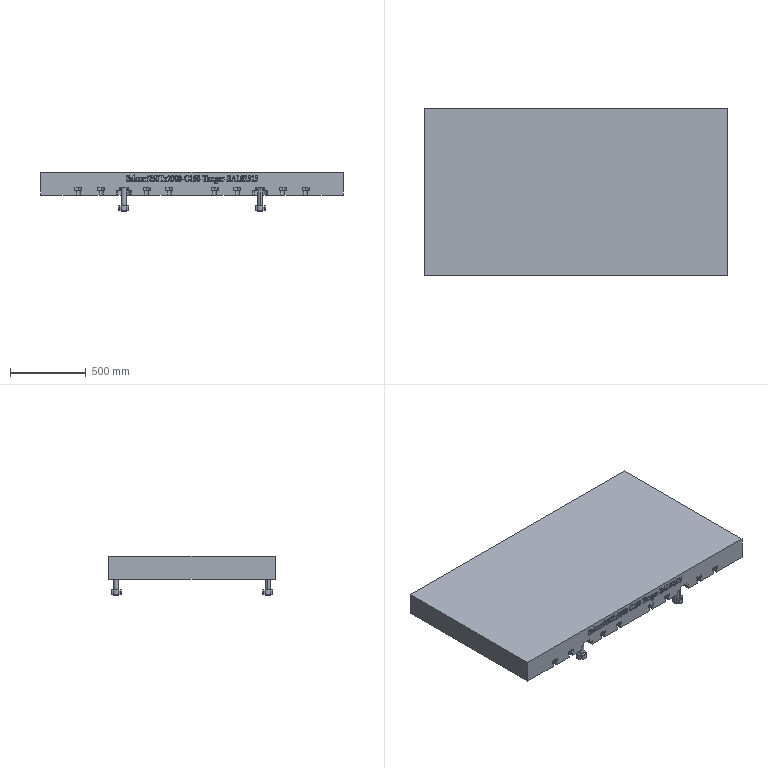Part | CATIA | 1 solid | 1044 faces | box 2000 x 1100 x 259.5 mm | volume 317583648 mm3 | plane 475 | other 410 | cylinder 127 | cone 32 | commonest cylinder face diameters 46 x40 28 x20 32 x16 56 x16 65 x16 100 x16